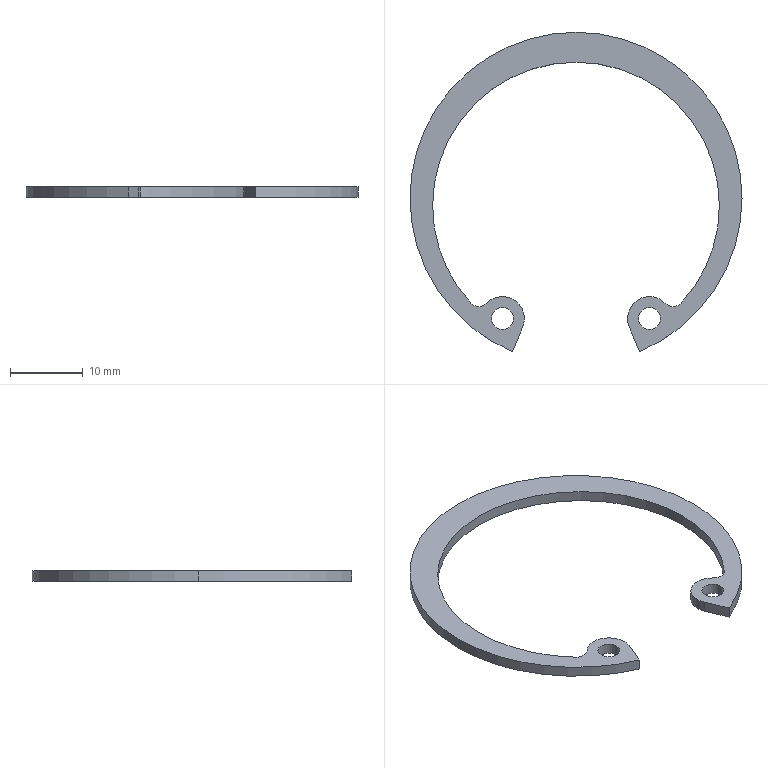Part | SolidWorks | features Extrusion 1 | 1 solid | 19 faces | box 45.5 x 43.768 x 1.5 mm | volume 608.831 mm3 | cylinder 15 | plane 4 | commonest cylinder face diameters 3 x6 6 x3 39.3 x3 45.5 x3
STEP:
#1=CARTESIAN_POINT('',(-11.568,-16.466,-1.5));
#2=VERTEX_POINT('',#1);
#3=CARTESIAN_POINT('',(-8.568,-16.466,-1.5));
#4=VERTEX_POINT('',#3);
#5=CARTESIAN_POINT('',(-10.068,-16.466,-1.5));
#6=DIRECTION('',(0.,0.,1.));
#7=DIRECTION('',(1.,0.,0.));
#8=AXIS2_PLACEMENT_3D('',#5,#6,#7);
#9=CIRCLE('',#8,1.5);
#10=EDGE_CURVE('',#2,#4,#9,.T.);
#11=ORIENTED_EDGE('',*,*,#10,.F.);
#12=CARTESIAN_POINT('',(-11.568,-16.466,0.));
#13=VERTEX_POINT('',#12);
#14=CARTESIAN_POINT('',(-11.568,-16.466,-1.5));
#15=DIRECTION('',(0.,0.,1.));
#16=VECTOR('',#15,1000.);
#17=LINE('',#14,#16);
#18=EDGE_CURVE('',#2,#13,#17,.T.);
#19=ORIENTED_EDGE('',*,*,#18,.T.);
#20=CARTESIAN_POINT('',(-8.568,-16.466,0.));
#21=VERTEX_POINT('',#20);
#22=CARTESIAN_POINT('',(-10.068,-16.466,0.));
#23=DIRECTION('',(0.,0.,1.));
#24=DIRECTION('',(1.,0.,0.));
#25=AXIS2_PLACEMENT_3D('',#22,#23,#24);
#26=CIRCLE('',#25,1.5);
#27=EDGE_CURVE('',#13,#21,#26,.T.);
#28=ORIENTED_EDGE('',*,*,#27,.T.);
#29=CARTESIAN_POINT('',(-8.568,-16.466,-1.5));
#30=DIRECTION('',(0.,0.,1.));
#31=VECTOR('',#30,1000.);
#32=LINE('',#29,#31);
#33=EDGE_CURVE('',#4,#21,#32,.T.);
#34=ORIENTED_EDGE('',*,*,#33,.F.);
#35=EDGE_LOOP('',(#11,#19,#28,#34));
#36=FACE_OUTER_BOUND('',#35,.T.);
#37=CARTESIAN_POINT('',(-10.068,-16.466,-1.5));
#38=DIRECTION('',(0.,0.,1.));
#39=DIRECTION('',(1.,0.,0.));
#40=AXIS2_PLACEMENT_3D('',#37,#38,#39);
#41=CYLINDRICAL_SURFACE('',#40,1.5);
#42=ADVANCED_FACE('',(#36),#41,.F.);
#43=CARTESIAN_POINT('',(8.568,-16.466,-1.5));
#44=VERTEX_POINT('',#43);
#45=CARTESIAN_POINT('',(11.568,-16.466,-1.5));
#46=VERTEX_POINT('',#45);
#47=CARTESIAN_POINT('',(10.068,-16.466,-1.5));
#48=DIRECTION('',(0.,0.,1.));
#49=DIRECTION('',(-1.,0.,0.));
#50=AXIS2_PLACEMENT_3D('',#47,#48,#49);
#51=CIRCLE('',#50,1.5);
#52=EDGE_CURVE('',#44,#46,#51,.T.);
#53=ORIENTED_EDGE('',*,*,#52,.F.);
#54=CARTESIAN_POINT('',(8.568,-16.466,0.));
#55=VERTEX_POINT('',#54);
#56=CARTESIAN_POINT('',(8.568,-16.466,-1.5));
#57=DIRECTION('',(0.,0.,1.));
#58=VECTOR('',#57,1000.);
#59=LINE('',#56,#58);
#60=EDGE_CURVE('',#44,#55,#59,.T.);
#61=ORIENTED_EDGE('',*,*,#60,.T.);
#62=CARTESIAN_POINT('',(11.568,-16.466,0.));
#63=VERTEX_POINT('',#62);
#64=CARTESIAN_POINT('',(10.068,-16.466,0.));
#65=DIRECTION('',(0.,0.,1.));
#66=DIRECTION('',(-1.,0.,0.));
#67=AXIS2_PLACEMENT_3D('',#64,#65,#66);
#68=CIRCLE('',#67,1.5);
#69=EDGE_CURVE('',#55,#63,#68,.T.);
#70=ORIENTED_EDGE('',*,*,#69,.T.);
#71=CARTESIAN_POINT('',(11.568,-16.466,-1.5));
#72=DIRECTION('',(0.,0.,1.));
#73=VECTOR('',#72,1000.);
#74=LINE('',#71,#73);
#75=EDGE_CURVE('',#46,#63,#74,.T.);
#76=ORIENTED_EDGE('',*,*,#75,.F.);
#77=EDGE_LOOP('',(#53,#61,#70,#76));
#78=FACE_OUTER_BOUND('',#77,.T.);
#79=CARTESIAN_POINT('',(10.068,-16.466,-1.5));
#80=DIRECTION('',(0.,0.,1.));
#81=DIRECTION('',(1.,0.,0.));
#82=AXIS2_PLACEMENT_3D('',#79,#80,#81);
#83=CYLINDRICAL_SURFACE('',#82,1.5);
#84=ADVANCED_FACE('',(#78),#83,.F.);
#85=CARTESIAN_POINT('',(-7.296,-17.614,-1.5));
#86=VERTEX_POINT('',#85);
#87=CARTESIAN_POINT('',(-7.068,-16.466,-1.5));
#88=VERTEX_POINT('',#87);
#89=CARTESIAN_POINT('',(-10.068,-16.466,-1.5));
#90=DIRECTION('',(0.,0.,1.));
#91=DIRECTION('',(1.,0.,0.));
#92=AXIS2_PLACEMENT_3D('',#89,#90,#91);
#93=CIRCLE('',#92,3.);
#94=EDGE_CURVE('',#86,#88,#93,.T.);
#95=ORIENTED_EDGE('',*,*,#94,.T.);
#96=CARTESIAN_POINT('',(-7.068,-16.466,0.));
#97=VERTEX_POINT('',#96);
#98=CARTESIAN_POINT('',(-7.068,-16.466,-1.5));
#99=DIRECTION('',(0.,0.,1.));
#100=VECTOR('',#99,1000.);
#101=LINE('',#98,#100);
#102=EDGE_CURVE('',#88,#97,#101,.T.);
#103=ORIENTED_EDGE('',*,*,#102,.T.);
#104=CARTESIAN_POINT('',(-7.296,-17.614,0.));
#105=VERTEX_POINT('',#104);
#106=CARTESIAN_POINT('',(-10.068,-16.466,0.));
#107=DIRECTION('',(0.,0.,1.));
#108=DIRECTION('',(1.,0.,0.));
#109=AXIS2_PLACEMENT_3D('',#106,#107,#108);
#110=CIRCLE('',#109,3.);
#111=EDGE_CURVE('',#105,#97,#110,.T.);
#112=ORIENTED_EDGE('',*,*,#111,.F.);
#113=CARTESIAN_POINT('',(-7.296,-17.614,-1.5));
#114=DIRECTION('',(0.,0.,1.));
#115=VECTOR('',#114,1000.);
#116=LINE('',#113,#115);
#117=EDGE_CURVE('',#86,#105,#116,.T.);
#118=ORIENTED_EDGE('',*,*,#117,.F.);
#119=EDGE_LOOP('',(#95,#103,#112,#118));
#120=FACE_OUTER_BOUND('',#119,.T.);
#121=CARTESIAN_POINT('',(-10.068,-16.466,-1.5));
#122=DIRECTION('',(0.,0.,1.));
#123=DIRECTION('',(1.,0.,0.));
#124=AXIS2_PLACEMENT_3D('',#121,#122,#123);
#125=CYLINDRICAL_SURFACE('',#124,3.);
#126=ADVANCED_FACE('',(#120),#125,.T.);
#127=CARTESIAN_POINT('',(-14.407,-14.363,-1.5));
#128=VERTEX_POINT('',#127);
#129=CARTESIAN_POINT('',(-19.65,-1.,-1.5));
#130=VERTEX_POINT('',#129);
#131=CARTESIAN_POINT('',(0.,-1.,-1.5));
#132=DIRECTION('',(0.,0.,-1.));
#133=DIRECTION('',(1.,0.,0.));
#134=AXIS2_PLACEMENT_3D('',#131,#132,#133);
#135=CIRCLE('',#134,19.65);
#136=EDGE_CURVE('',#128,#130,#135,.T.);
#137=ORIENTED_EDGE('',*,*,#136,.T.);
#138=CARTESIAN_POINT('',(-19.65,-1.,0.));
#139=VERTEX_POINT('',#138);
#140=CARTESIAN_POINT('',(-19.65,-1.,-1.5));
#141=DIRECTION('',(0.,0.,1.));
#142=VECTOR('',#141,1000.);
#143=LINE('',#140,#142);
#144=EDGE_CURVE('',#130,#139,#143,.T.);
#145=ORIENTED_EDGE('',*,*,#144,.T.);
#146=CARTESIAN_POINT('',(-14.407,-14.363,0.));
#147=VERTEX_POINT('',#146);
#148=CARTESIAN_POINT('',(0.,-1.,0.));
#149=DIRECTION('',(0.,0.,-1.));
#150=DIRECTION('',(1.,0.,0.));
#151=AXIS2_PLACEMENT_3D('',#148,#149,#150);
#152=CIRCLE('',#151,19.65);
#153=EDGE_CURVE('',#147,#139,#152,.T.);
#154=ORIENTED_EDGE('',*,*,#153,.F.);
#155=CARTESIAN_POINT('',(-14.407,-14.363,-1.5));
#156=DIRECTION('',(0.,0.,1.));
#157=VECTOR('',#156,1000.);
#158=LINE('',#155,#157);
#159=EDGE_CURVE('',#128,#147,#158,.T.);
#160=ORIENTED_EDGE('',*,*,#159,.F.);
#161=EDGE_LOOP('',(#137,#145,#154,#160));
#162=FACE_OUTER_BOUND('',#161,.T.);
#163=CARTESIAN_POINT('',(0.,-1.,-1.5));
#164=DIRECTION('',(0.,0.,1.));
#165=DIRECTION('',(1.,0.,0.));
#166=AXIS2_PLACEMENT_3D('',#163,#164,#165);
#167=CYLINDRICAL_SURFACE('',#166,19.65);
#168=ADVANCED_FACE('',(#162),#167,.F.);
#169=ORIENTED_EDGE('',*,*,#144,.F.);
#170=CARTESIAN_POINT('',(19.65,-1.,-1.5));
#171=VERTEX_POINT('',#170);
#172=CARTESIAN_POINT('',(0.,-1.,-1.5));
#173=DIRECTION('',(0.,0.,-1.));
#174=DIRECTION('',(1.,0.,0.));
#175=AXIS2_PLACEMENT_3D('',#172,#173,#174);
#176=CIRCLE('',#175,19.65);
#177=EDGE_CURVE('',#130,#171,#176,.T.);
#178=ORIENTED_EDGE('',*,*,#177,.T.);
#179=CARTESIAN_POINT('',(19.65,-1.,0.));
#180=VERTEX_POINT('',#179);
#181=CARTESIAN_POINT('',(19.65,-1.,-1.5));
#182=DIRECTION('',(0.,0.,1.));
#183=VECTOR('',#182,1000.);
#184=LINE('',#181,#183);
#185=EDGE_CURVE('',#171,#180,#184,.T.);
#186=ORIENTED_EDGE('',*,*,#185,.T.);
#187=CARTESIAN_POINT('',(0.,-1.,0.));
#188=DIRECTION('',(0.,0.,-1.));
#189=DIRECTION('',(1.,0.,0.));
#190=AXIS2_PLACEMENT_3D('',#187,#188,#189);
#191=CIRCLE('',#190,19.65);
#192=EDGE_CURVE('',#139,#180,#191,.T.);
#193=ORIENTED_EDGE('',*,*,#192,.F.);
#194=EDGE_LOOP('',(#169,#178,#186,#193));
#195=FACE_OUTER_BOUND('',#194,.T.);
#196=CARTESIAN_POINT('',(0.,-1.,-1.5));
#197=DIRECTION('',(0.,0.,1.));
#198=DIRECTION('',(1.,0.,0.));
#199=AXIS2_PLACEMENT_3D('',#196,#197,#198);
#200=CYLINDRICAL_SURFACE('',#199,19.65);
#201=ADVANCED_FACE('',(#195),#200,.F.);
#202=CARTESIAN_POINT('',(22.75,0.,-1.5));
#203=VERTEX_POINT('',#202);
#204=CARTESIAN_POINT('',(-22.75,0.,-1.5));
#205=VERTEX_POINT('',#204);
#206=CARTESIAN_POINT('',(0.,0.,-1.5));
#207=DIRECTION('',(0.,0.,1.));
#208=DIRECTION('',(1.,0.,0.));
#209=AXIS2_PLACEMENT_3D('',#206,#207,#208);
#210=CIRCLE('',#209,22.75);
#211=EDGE_CURVE('',#203,#205,#210,.T.);
#212=ORIENTED_EDGE('',*,*,#211,.T.);
#213=CARTESIAN_POINT('',(-22.75,0.,0.));
#214=VERTEX_POINT('',#213);
#215=CARTESIAN_POINT('',(-22.75,0.,-1.5));
#216=DIRECTION('',(0.,0.,1.));
#217=VECTOR('',#216,1000.);
#218=LINE('',#215,#217);
#219=EDGE_CURVE('',#205,#214,#218,.T.);
#220=ORIENTED_EDGE('',*,*,#219,.T.);
#221=CARTESIAN_POINT('',(22.75,0.,0.));
#222=VERTEX_POINT('',#221);
#223=CARTESIAN_POINT('',(0.,0.,0.));
#224=DIRECTION('',(0.,0.,1.));
#225=DIRECTION('',(1.,0.,0.));
#226=AXIS2_PLACEMENT_3D('',#223,#224,#225);
#227=CIRCLE('',#226,22.75);
#228=EDGE_CURVE('',#222,#214,#227,.T.);
#229=ORIENTED_EDGE('',*,*,#228,.F.);
#230=CARTESIAN_POINT('',(22.75,0.,-1.5));
#231=DIRECTION('',(0.,0.,1.));
#232=VECTOR('',#231,1000.);
#233=LINE('',#230,#232);
#234=EDGE_CURVE('',#203,#222,#233,.T.);
#235=ORIENTED_EDGE('',*,*,#234,.F.);
#236=EDGE_LOOP('',(#212,#220,#229,#235));
#237=FACE_OUTER_BOUND('',#236,.T.);
#238=CARTESIAN_POINT('',(0.,0.,-1.5));
#239=DIRECTION('',(0.,0.,1.));
#240=DIRECTION('',(1.,0.,0.));
#241=AXIS2_PLACEMENT_3D('',#238,#239,#240);
#242=CYLINDRICAL_SURFACE('',#241,22.75);
#243=ADVANCED_FACE('',(#237),#242,.T.);
#244=CARTESIAN_POINT('',(8.706,-21.018,-1.5));
#245=VERTEX_POINT('',#244);
#246=CARTESIAN_POINT('',(0.,0.,-1.5));
#247=DIRECTION('',(0.,0.,1.));
#248=DIRECTION('',(1.,0.,0.));
#249=AXIS2_PLACEMENT_3D('',#246,#247,#248);
#250=CIRCLE('',#249,22.75);
#251=EDGE_CURVE('',#245,#203,#250,.T.);
#252=ORIENTED_EDGE('',*,*,#251,.T.);
#253=ORIENTED_EDGE('',*,*,#234,.T.);
#254=CARTESIAN_POINT('',(8.706,-21.018,0.));
#255=VERTEX_POINT('',#254);
#256=CARTESIAN_POINT('',(0.,0.,0.));
#257=DIRECTION('',(0.,0.,1.));
#258=DIRECTION('',(1.,0.,0.));
#259=AXIS2_PLACEMENT_3D('',#256,#257,#258);
#260=CIRCLE('',#259,22.75);
#261=EDGE_CURVE('',#255,#222,#260,.T.);
#262=ORIENTED_EDGE('',*,*,#261,.F.);
#263=CARTESIAN_POINT('',(8.706,-21.018,-1.5));
#264=DIRECTION('',(0.,0.,1.));
#265=VECTOR('',#264,1000.);
#266=LINE('',#263,#265);
#267=EDGE_CURVE('',#245,#255,#266,.T.);
#268=ORIENTED_EDGE('',*,*,#267,.F.);
#269=EDGE_LOOP('',(#252,#253,#262,#268));
#270=FACE_OUTER_BOUND('',#269,.T.);
#271=CARTESIAN_POINT('',(0.,0.,-1.5));
#272=DIRECTION('',(0.,0.,1.));
#273=DIRECTION('',(1.,0.,0.));
#274=AXIS2_PLACEMENT_3D('',#271,#272,#273);
#275=CYLINDRICAL_SURFACE('',#274,22.75);
#276=ADVANCED_FACE('',(#270),#275,.T.);
#277=ORIENTED_EDGE('',*,*,#219,.F.);
#278=CARTESIAN_POINT('',(-8.706,-21.018,-1.5));
#279=VERTEX_POINT('',#278);
#280=CARTESIAN_POINT('',(0.,0.,-1.5));
#281=DIRECTION('',(0.,0.,1.));
#282=DIRECTION('',(1.,0.,0.));
#283=AXIS2_PLACEMENT_3D('',#280,#281,#282);
#284=CIRCLE('',#283,22.75);
#285=EDGE_CURVE('',#205,#279,#284,.T.);
#286=ORIENTED_EDGE('',*,*,#285,.T.);
#287=CARTESIAN_POINT('',(-8.706,-21.018,0.));
#288=VERTEX_POINT('',#287);
#289=CARTESIAN_POINT('',(-8.706,-21.018,-1.5));
#290=DIRECTION('',(0.,0.,1.));
#291=VECTOR('',#290,1000.);
#292=LINE('',#289,#291);
#293=EDGE_CURVE('',#279,#288,#292,.T.);
#294=ORIENTED_EDGE('',*,*,#293,.T.);
#295=CARTESIAN_POINT('',(0.,0.,0.));
#296=DIRECTION('',(0.,0.,1.));
#297=DIRECTION('',(1.,0.,0.));
#298=AXIS2_PLACEMENT_3D('',#295,#296,#297);
#299=CIRCLE('',#298,22.75);
#300=EDGE_CURVE('',#214,#288,#299,.T.);
#301=ORIENTED_EDGE('',*,*,#300,.F.);
#302=EDGE_LOOP('',(#277,#286,#294,#301));
#303=FACE_OUTER_BOUND('',#302,.T.);
#304=CARTESIAN_POINT('',(0.,0.,-1.5));
#305=DIRECTION('',(0.,0.,1.));
#306=DIRECTION('',(1.,0.,0.));
#307=AXIS2_PLACEMENT_3D('',#304,#305,#306);
#308=CYLINDRICAL_SURFACE('',#307,22.75);
#309=ADVANCED_FACE('',(#303),#308,.T.);
#310=CARTESIAN_POINT('',(7.296,-17.614,0.));
#311=VERTEX_POINT('',#310);
#312=CARTESIAN_POINT('',(7.296,-17.614,0.));
#313=DIRECTION('',(0.3827,-0.9239,0.));
#314=VECTOR('',#313,1000.);
#315=LINE('',#312,#314);
#316=EDGE_CURVE('',#311,#255,#315,.T.);
#317=ORIENTED_EDGE('',*,*,#316,.F.);
#318=CARTESIAN_POINT('',(7.296,-17.614,-1.5));
#319=VERTEX_POINT('',#318);
#320=CARTESIAN_POINT('',(7.296,-17.614,-1.5));
#321=DIRECTION('',(0.,0.,1.));
#322=VECTOR('',#321,1000.);
#323=LINE('',#320,#322);
#324=EDGE_CURVE('',#319,#311,#323,.T.);
#325=ORIENTED_EDGE('',*,*,#324,.F.);
#326=CARTESIAN_POINT('',(7.296,-17.614,-1.5));
#327=DIRECTION('',(0.3827,-0.9239,0.));
#328=VECTOR('',#327,1000.);
#329=LINE('',#326,#328);
#330=EDGE_CURVE('',#319,#245,#329,.T.);
#331=ORIENTED_EDGE('',*,*,#330,.T.);
#332=ORIENTED_EDGE('',*,*,#267,.T.);
#333=EDGE_LOOP('',(#317,#325,#331,#332));
#334=FACE_OUTER_BOUND('',#333,.T.);
#335=CARTESIAN_POINT('',(7.296,-17.614,-1.5));
#336=DIRECTION('',(-0.9239,-0.3827,0.));
#337=DIRECTION('',(0.3827,-0.9239,0.));
#338=AXIS2_PLACEMENT_3D('',#335,#336,#337);
#339=PLANE('',#338);
#340=ADVANCED_FACE('',(#334),#339,.T.);
#341=CARTESIAN_POINT('',(12.227,-14.384,0.));
#342=VERTEX_POINT('',#341);
#343=CARTESIAN_POINT('',(10.068,-16.466,0.));
#344=DIRECTION('',(0.,0.,1.));
#345=DIRECTION('',(-1.,0.,0.));
#346=AXIS2_PLACEMENT_3D('',#343,#344,#345);
#347=CIRCLE('',#346,3.);
#348=EDGE_CURVE('',#342,#311,#347,.T.);
#349=ORIENTED_EDGE('',*,*,#348,.F.);
#350=CARTESIAN_POINT('',(12.227,-14.384,-1.5));
#351=VERTEX_POINT('',#350);
#352=CARTESIAN_POINT('',(12.227,-14.384,-1.5));
#353=DIRECTION('',(0.,0.,1.));
#354=VECTOR('',#353,1000.);
#355=LINE('',#352,#354);
#356=EDGE_CURVE('',#351,#342,#355,.T.);
#357=ORIENTED_EDGE('',*,*,#356,.F.);
#358=CARTESIAN_POINT('',(10.068,-16.466,-1.5));
#359=DIRECTION('',(0.,0.,1.));
#360=DIRECTION('',(-1.,0.,0.));
#361=AXIS2_PLACEMENT_3D('',#358,#359,#360);
#362=CIRCLE('',#361,3.);
#363=EDGE_CURVE('',#351,#319,#362,.T.);
#364=ORIENTED_EDGE('',*,*,#363,.T.);
#365=ORIENTED_EDGE('',*,*,#324,.T.);
#366=EDGE_LOOP('',(#349,#357,#364,#365));
#367=FACE_OUTER_BOUND('',#366,.T.);
#368=CARTESIAN_POINT('',(10.068,-16.466,-1.5));
#369=DIRECTION('',(0.,0.,1.));
#370=DIRECTION('',(1.,0.,0.));
#371=AXIS2_PLACEMENT_3D('',#368,#369,#370);
#372=CYLINDRICAL_SURFACE('',#371,3.);
#373=ADVANCED_FACE('',(#367),#372,.T.);
#374=CARTESIAN_POINT('',(14.407,-14.363,0.));
#375=VERTEX_POINT('',#374);
#376=CARTESIAN_POINT('',(13.307,-13.343,0.));
#377=DIRECTION('',(0.,0.,-1.));
#378=DIRECTION('',(-1.,0.,0.));
#379=AXIS2_PLACEMENT_3D('',#376,#377,#378);
#380=CIRCLE('',#379,1.5);
#381=EDGE_CURVE('',#375,#342,#380,.T.);
#382=ORIENTED_EDGE('',*,*,#381,.F.);
#383=CARTESIAN_POINT('',(14.407,-14.363,-1.5));
#384=VERTEX_POINT('',#383);
#385=CARTESIAN_POINT('',(14.407,-14.363,-1.5));
#386=DIRECTION('',(0.,0.,1.));
#387=VECTOR('',#386,1000.);
#388=LINE('',#385,#387);
#389=EDGE_CURVE('',#384,#375,#388,.T.);
#390=ORIENTED_EDGE('',*,*,#389,.F.);
#391=CARTESIAN_POINT('',(13.307,-13.343,-1.5));
#392=DIRECTION('',(0.,0.,-1.));
#393=DIRECTION('',(-1.,0.,0.));
#394=AXIS2_PLACEMENT_3D('',#391,#392,#393);
#395=CIRCLE('',#394,1.5);
#396=EDGE_CURVE('',#384,#351,#395,.T.);
#397=ORIENTED_EDGE('',*,*,#396,.T.);
#398=ORIENTED_EDGE('',*,*,#356,.T.);
#399=EDGE_LOOP('',(#382,#390,#397,#398));
#400=FACE_OUTER_BOUND('',#399,.T.);
#401=CARTESIAN_POINT('',(13.307,-13.343,-1.5));
#402=DIRECTION('',(0.,0.,1.));
#403=DIRECTION('',(1.,0.,0.));
#404=AXIS2_PLACEMENT_3D('',#401,#402,#403);
#405=CYLINDRICAL_SURFACE('',#404,1.5);
#406=ADVANCED_FACE('',(#400),#405,.F.);
#407=ORIENTED_EDGE('',*,*,#185,.F.);
#408=CARTESIAN_POINT('',(0.,-1.,-1.5));
#409=DIRECTION('',(0.,0.,-1.));
#410=DIRECTION('',(1.,0.,0.));
#411=AXIS2_PLACEMENT_3D('',#408,#409,#410);
#412=CIRCLE('',#411,19.65);
#413=EDGE_CURVE('',#171,#384,#412,.T.);
#414=ORIENTED_EDGE('',*,*,#413,.T.);
#415=ORIENTED_EDGE('',*,*,#389,.T.);
#416=CARTESIAN_POINT('',(0.,-1.,0.));
#417=DIRECTION('',(0.,0.,-1.));
#418=DIRECTION('',(1.,0.,0.));
#419=AXIS2_PLACEMENT_3D('',#416,#417,#418);
#420=CIRCLE('',#419,19.65);
#421=EDGE_CURVE('',#180,#375,#420,.T.);
#422=ORIENTED_EDGE('',*,*,#421,.F.);
#423=EDGE_LOOP('',(#407,#414,#415,#422));
#424=FACE_OUTER_BOUND('',#423,.T.);
#425=CARTESIAN_POINT('',(0.,-1.,-1.5));
#426=DIRECTION('',(0.,0.,1.));
#427=DIRECTION('',(1.,0.,0.));
#428=AXIS2_PLACEMENT_3D('',#425,#426,#427);
#429=CYLINDRICAL_SURFACE('',#428,19.65);
#430=ADVANCED_FACE('',(#424),#429,.F.);
#431=CARTESIAN_POINT('',(-12.227,-14.384,0.));
#432=VERTEX_POINT('',#431);
#433=CARTESIAN_POINT('',(-13.307,-13.343,0.));
#434=DIRECTION('',(0.,0.,-1.));
#435=DIRECTION('',(1.,0.,0.));
#436=AXIS2_PLACEMENT_3D('',#433,#434,#435);
#437=CIRCLE('',#436,1.5);
#438=EDGE_CURVE('',#432,#147,#437,.T.);
#439=ORIENTED_EDGE('',*,*,#438,.F.);
#440=CARTESIAN_POINT('',(-12.227,-14.384,-1.5));
#441=VERTEX_POINT('',#440);
#442=CARTESIAN_POINT('',(-12.227,-14.384,-1.5));
#443=DIRECTION('',(0.,0.,1.));
#444=VECTOR('',#443,1000.);
#445=LINE('',#442,#444);
#446=EDGE_CURVE('',#441,#432,#445,.T.);
#447=ORIENTED_EDGE('',*,*,#446,.F.);
#448=CARTESIAN_POINT('',(-13.307,-13.343,-1.5));
#449=DIRECTION('',(0.,0.,-1.));
#450=DIRECTION('',(1.,0.,0.));
#451=AXIS2_PLACEMENT_3D('',#448,#449,#450);
#452=CIRCLE('',#451,1.5);
#453=EDGE_CURVE('',#441,#128,#452,.T.);
#454=ORIENTED_EDGE('',*,*,#453,.T.);
#455=ORIENTED_EDGE('',*,*,#159,.T.);
#456=EDGE_LOOP('',(#439,#447,#454,#455));
#457=FACE_OUTER_BOUND('',#456,.T.);
#458=CARTESIAN_POINT('',(-13.307,-13.343,-1.5));
#459=DIRECTION('',(0.,0.,1.));
#460=DIRECTION('',(1.,0.,0.));
#461=AXIS2_PLACEMENT_3D('',#458,#459,#460);
#462=CYLINDRICAL_SURFACE('',#461,1.5);
#463=ADVANCED_FACE('',(#457),#462,.F.);
#464=ORIENTED_EDGE('',*,*,#102,.F.);
#465=CARTESIAN_POINT('',(-10.068,-16.466,-1.5));
#466=DIRECTION('',(0.,0.,1.));
#467=DIRECTION('',(1.,0.,0.));
#468=AXIS2_PLACEMENT_3D('',#465,#466,#467);
#469=CIRCLE('',#468,3.);
#470=EDGE_CURVE('',#88,#441,#469,.T.);
#471=ORIENTED_EDGE('',*,*,#470,.T.);
#472=ORIENTED_EDGE('',*,*,#446,.T.);
#473=CARTESIAN_POINT('',(-10.068,-16.466,0.));
#474=DIRECTION('',(0.,0.,1.));
#475=DIRECTION('',(1.,0.,0.));
#476=AXIS2_PLACEMENT_3D('',#473,#474,#475);
#477=CIRCLE('',#476,3.);
#478=EDGE_CURVE('',#97,#432,#477,.T.);
#479=ORIENTED_EDGE('',*,*,#478,.F.);
#480=EDGE_LOOP('',(#464,#471,#472,#479));
#481=FACE_OUTER_BOUND('',#480,.T.);
#482=CARTESIAN_POINT('',(-10.068,-16.466,-1.5));
#483=DIRECTION('',(0.,0.,1.));
#484=DIRECTION('',(1.,0.,0.));
#485=AXIS2_PLACEMENT_3D('',#482,#483,#484);
#486=CYLINDRICAL_SURFACE('',#485,3.);
#487=ADVANCED_FACE('',(#481),#486,.T.);
#488=CARTESIAN_POINT('',(-7.296,-17.614,0.));
#489=DIRECTION('',(0.3827,0.9239,0.));
#490=VECTOR('',#489,1000.);
#491=LINE('',#488,#490);
#492=EDGE_CURVE('',#288,#105,#491,.T.);
#493=ORIENTED_EDGE('',*,*,#492,.F.);
#494=ORIENTED_EDGE('',*,*,#293,.F.);
#495=CARTESIAN_POINT('',(-7.296,-17.614,-1.5));
#496=DIRECTION('',(0.3827,0.9239,0.));
#497=VECTOR('',#496,1000.);
#498=LINE('',#495,#497);
#499=EDGE_CURVE('',#279,#86,#498,.T.);
#500=ORIENTED_EDGE('',*,*,#499,.T.);
#501=ORIENTED_EDGE('',*,*,#117,.T.);
#502=EDGE_LOOP('',(#493,#494,#500,#501));
#503=FACE_OUTER_BOUND('',#502,.T.);
#504=CARTESIAN_POINT('',(-7.296,-17.614,-1.5));
#505=DIRECTION('',(0.9239,-0.3827,0.));
#506=DIRECTION('',(0.3827,0.9239,0.));
#507=AXIS2_PLACEMENT_3D('',#504,#505,#506);
#508=PLANE('',#507);
#509=ADVANCED_FACE('',(#503),#508,.T.);
#510=CARTESIAN_POINT('',(-10.068,-16.466,-1.5));
#511=DIRECTION('',(0.,0.,1.));
#512=DIRECTION('',(1.,0.,0.));
#513=AXIS2_PLACEMENT_3D('',#510,#511,#512);
#514=CIRCLE('',#513,1.5);
#515=EDGE_CURVE('',#4,#2,#514,.T.);
#516=ORIENTED_EDGE('',*,*,#515,.T.);
#517=ORIENTED_EDGE('',*,*,#10,.T.);
#518=EDGE_LOOP('',(#516,#517));
#519=FACE_BOUND('',#518,.T.);
#520=CARTESIAN_POINT('',(10.068,-16.466,-1.5));
#521=DIRECTION('',(0.,0.,1.));
#522=DIRECTION('',(-1.,0.,0.));
#523=AXIS2_PLACEMENT_3D('',#520,#521,#522);
#524=CIRCLE('',#523,1.5);
#525=EDGE_CURVE('',#46,#44,#524,.T.);
#526=ORIENTED_EDGE('',*,*,#525,.T.);
#527=ORIENTED_EDGE('',*,*,#52,.T.);
#528=EDGE_LOOP('',(#526,#527));
#529=FACE_BOUND('',#528,.T.);
#530=ORIENTED_EDGE('',*,*,#251,.F.);
#531=ORIENTED_EDGE('',*,*,#330,.F.);
#532=ORIENTED_EDGE('',*,*,#363,.F.);
#533=ORIENTED_EDGE('',*,*,#396,.F.);
#534=ORIENTED_EDGE('',*,*,#413,.F.);
#535=ORIENTED_EDGE('',*,*,#177,.F.);
#536=ORIENTED_EDGE('',*,*,#136,.F.);
#537=ORIENTED_EDGE('',*,*,#453,.F.);
#538=ORIENTED_EDGE('',*,*,#470,.F.);
#539=ORIENTED_EDGE('',*,*,#94,.F.);
#540=ORIENTED_EDGE('',*,*,#499,.F.);
#541=ORIENTED_EDGE('',*,*,#285,.F.);
#542=ORIENTED_EDGE('',*,*,#211,.F.);
#543=EDGE_LOOP('',(#530,#531,#532,#533,#534,#535,#536,#537,#538,#539,#540,#541,#542));
#544=FACE_OUTER_BOUND('',#543,.T.);
#545=CARTESIAN_POINT('',(0.,0.,-1.5));
#546=DIRECTION('',(0.,0.,1.));
#547=DIRECTION('',(1.,0.,0.));
#548=AXIS2_PLACEMENT_3D('',#545,#546,#547);
#549=PLANE('',#548);
#550=ADVANCED_FACE('',(#519,#529,#544),#549,.F.);
#551=CARTESIAN_POINT('',(-10.068,-16.466,0.));
#552=DIRECTION('',(0.,0.,1.));
#553=DIRECTION('',(1.,0.,0.));
#554=AXIS2_PLACEMENT_3D('',#551,#552,#553);
#555=CIRCLE('',#554,1.5);
#556=EDGE_CURVE('',#21,#13,#555,.T.);
#557=ORIENTED_EDGE('',*,*,#556,.F.);
#558=ORIENTED_EDGE('',*,*,#27,.F.);
#559=EDGE_LOOP('',(#557,#558));
#560=FACE_BOUND('',#559,.T.);
#561=CARTESIAN_POINT('',(10.068,-16.466,0.));
#562=DIRECTION('',(0.,0.,1.));
#563=DIRECTION('',(-1.,0.,0.));
#564=AXIS2_PLACEMENT_3D('',#561,#562,#563);
#565=CIRCLE('',#564,1.5);
#566=EDGE_CURVE('',#63,#55,#565,.T.);
#567=ORIENTED_EDGE('',*,*,#566,.F.);
#568=ORIENTED_EDGE('',*,*,#69,.F.);
#569=EDGE_LOOP('',(#567,#568));
#570=FACE_BOUND('',#569,.T.);
#571=ORIENTED_EDGE('',*,*,#261,.T.);
#572=ORIENTED_EDGE('',*,*,#228,.T.);
#573=ORIENTED_EDGE('',*,*,#300,.T.);
#574=ORIENTED_EDGE('',*,*,#492,.T.);
#575=ORIENTED_EDGE('',*,*,#111,.T.);
#576=ORIENTED_EDGE('',*,*,#478,.T.);
#577=ORIENTED_EDGE('',*,*,#438,.T.);
#578=ORIENTED_EDGE('',*,*,#153,.T.);
#579=ORIENTED_EDGE('',*,*,#192,.T.);
#580=ORIENTED_EDGE('',*,*,#421,.T.);
#581=ORIENTED_EDGE('',*,*,#381,.T.);
#582=ORIENTED_EDGE('',*,*,#348,.T.);
#583=ORIENTED_EDGE('',*,*,#316,.T.);
#584=EDGE_LOOP('',(#571,#572,#573,#574,#575,#576,#577,#578,#579,#580,#581,#582,#583));
#585=FACE_OUTER_BOUND('',#584,.T.);
#586=CARTESIAN_POINT('',(0.,0.,0.));
#587=DIRECTION('',(0.,0.,1.));
#588=DIRECTION('',(1.,0.,0.));
#589=AXIS2_PLACEMENT_3D('',#586,#587,#588);
#590=PLANE('',#589);
#591=ADVANCED_FACE('',(#560,#570,#585),#590,.T.);
#592=ORIENTED_EDGE('',*,*,#60,.F.);
#593=ORIENTED_EDGE('',*,*,#525,.F.);
#594=ORIENTED_EDGE('',*,*,#75,.T.);
#595=ORIENTED_EDGE('',*,*,#566,.T.);
#596=EDGE_LOOP('',(#592,#593,#594,#595));
#597=FACE_OUTER_BOUND('',#596,.T.);
#598=CARTESIAN_POINT('',(10.068,-16.466,-1.5));
#599=DIRECTION('',(0.,0.,1.));
#600=DIRECTION('',(1.,0.,0.));
#601=AXIS2_PLACEMENT_3D('',#598,#599,#600);
#602=CYLINDRICAL_SURFACE('',#601,1.5);
#603=ADVANCED_FACE('',(#597),#602,.F.);
#604=ORIENTED_EDGE('',*,*,#18,.F.);
#605=ORIENTED_EDGE('',*,*,#515,.F.);
#606=ORIENTED_EDGE('',*,*,#33,.T.);
#607=ORIENTED_EDGE('',*,*,#556,.T.);
#608=EDGE_LOOP('',(#604,#605,#606,#607));
#609=FACE_OUTER_BOUND('',#608,.T.);
#610=CARTESIAN_POINT('',(-10.068,-16.466,-1.5));
#611=DIRECTION('',(0.,0.,1.));
#612=DIRECTION('',(1.,0.,0.));
#613=AXIS2_PLACEMENT_3D('',#610,#611,#612);
#614=CYLINDRICAL_SURFACE('',#613,1.5);
#615=ADVANCED_FACE('',(#609),#614,.F.);
#616=CLOSED_SHELL('',(#42,#84,#126,#168,#201,#243,#276,#309,#340,#373,#406,#430,#463,#487,#509,#550,#591,#603,#615));
#617=MANIFOLD_SOLID_BREP('',#616);
#618=CARTESIAN_POINT('',(0.,0.,0.));
#619=DIRECTION('',(0.,0.,1.));
#620=DIRECTION('',(1.,0.,0.));
#621=AXIS2_PLACEMENT_3D('',#618,#619,#620);
#622=(LENGTH_UNIT()NAMED_UNIT(*)SI_UNIT(.MILLI.,.METRE.));
#623=UNCERTAINTY_MEASURE_WITH_UNIT(LENGTH_MEASURE(0.00001),#622,'','');
#624=(NAMED_UNIT(*)PLANE_ANGLE_UNIT()SI_UNIT($,.RADIAN.));
#625=(NAMED_UNIT(*)SI_UNIT($,.STERADIAN.)SOLID_ANGLE_UNIT());
#626=(GEOMETRIC_REPRESENTATION_CONTEXT(3)GLOBAL_UNCERTAINTY_ASSIGNED_CONTEXT((#623))GLOBAL_UNIT_ASSIGNED_CONTEXT((#622,#624,#625))REPRESENTATION_CONTEXT('',''));
#627=ADVANCED_BREP_SHAPE_REPRESENTATION('',(#617,#621),#626);